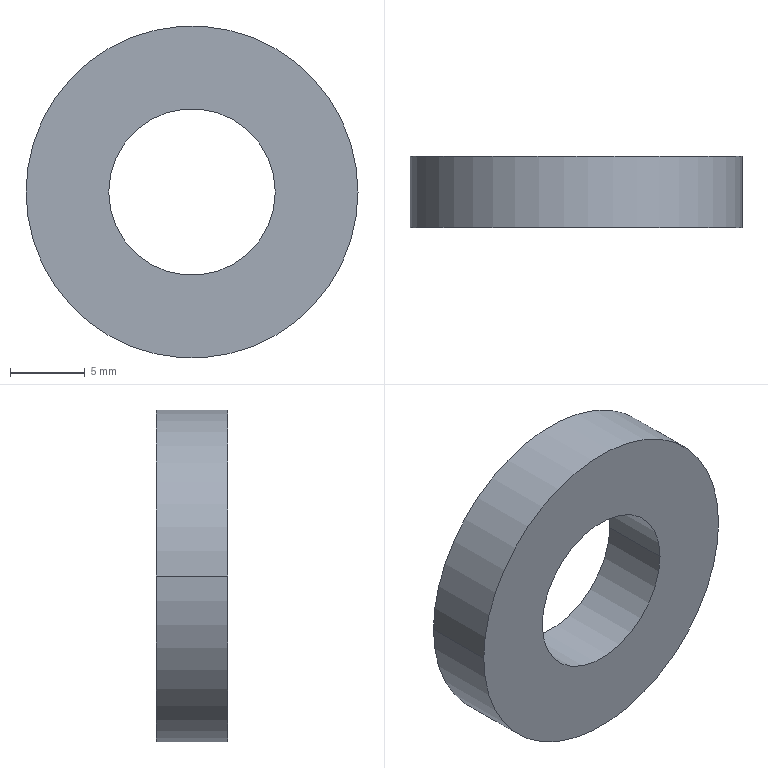Part | NX | features BREP 1 | 1 solid | 6 faces | box 22.225 x 4.763 x 22.225 mm | volume 1383 mm3 | cylinder 4 | plane 2 | commonest cylinder face diameters 11.151 x2 22.225 x2
STEP:
#1=CARTESIAN_POINT('',(-11.113,0.,0.));
#2=VERTEX_POINT('',#1);
#3=CARTESIAN_POINT('',(11.113,0.,0.));
#4=VERTEX_POINT('',#3);
#5=CARTESIAN_POINT('',(0.,0.,0.));
#6=DIRECTION('',(0.,1.,0.));
#7=DIRECTION('',(-1.,0.,0.));
#8=AXIS2_PLACEMENT_3D('',#5,#6,#7);
#9=CIRCLE('',#8,11.113);
#10=EDGE_CURVE('',#2,#4,#9,.T.);
#11=ORIENTED_EDGE('',*,*,#10,.F.);
#12=CARTESIAN_POINT('',(0.,0.,0.));
#13=DIRECTION('',(0.,1.,0.));
#14=DIRECTION('',(1.,0.,0.));
#15=AXIS2_PLACEMENT_3D('',#12,#13,#14);
#16=CIRCLE('',#15,11.113);
#17=EDGE_CURVE('',#4,#2,#16,.T.);
#18=ORIENTED_EDGE('',*,*,#17,.F.);
#19=EDGE_LOOP('',(#11,#18));
#20=FACE_BOUND('',#19,.T.);
#21=CARTESIAN_POINT('',(-5.575,0.,0.));
#22=VERTEX_POINT('',#21);
#23=CARTESIAN_POINT('',(5.575,0.,0.));
#24=VERTEX_POINT('',#23);
#25=CARTESIAN_POINT('',(0.,0.,0.));
#26=DIRECTION('',(0.,-1.,0.));
#27=DIRECTION('',(-1.,0.,0.));
#28=AXIS2_PLACEMENT_3D('',#25,#26,#27);
#29=CIRCLE('',#28,5.575);
#30=EDGE_CURVE('',#22,#24,#29,.T.);
#31=ORIENTED_EDGE('',*,*,#30,.F.);
#32=CARTESIAN_POINT('',(0.,0.,0.));
#33=DIRECTION('',(0.,-1.,0.));
#34=DIRECTION('',(1.,0.,0.));
#35=AXIS2_PLACEMENT_3D('',#32,#33,#34);
#36=CIRCLE('',#35,5.575);
#37=EDGE_CURVE('',#24,#22,#36,.T.);
#38=ORIENTED_EDGE('',*,*,#37,.F.);
#39=EDGE_LOOP('',(#31,#38));
#40=FACE_BOUND('',#39,.T.);
#41=CARTESIAN_POINT('',(0.,0.,0.));
#42=DIRECTION('',(0.,1.,0.));
#43=DIRECTION('',(1.,0.,0.));
#44=AXIS2_PLACEMENT_3D('',#41,#42,#43);
#45=PLANE('',#44);
#46=ADVANCED_FACE('',(#20,#40),#45,.F.);
#47=CARTESIAN_POINT('',(-11.113,4.763,0.));
#48=VERTEX_POINT('',#47);
#49=CARTESIAN_POINT('',(-11.113,0.,0.));
#50=DIRECTION('',(0.,1.,0.));
#51=VECTOR('',#50,1000.);
#52=LINE('',#49,#51);
#53=EDGE_CURVE('',#2,#48,#52,.T.);
#54=ORIENTED_EDGE('',*,*,#53,.T.);
#55=CARTESIAN_POINT('',(11.113,4.763,0.));
#56=VERTEX_POINT('',#55);
#57=CARTESIAN_POINT('',(0.,4.763,0.));
#58=DIRECTION('',(0.,1.,0.));
#59=DIRECTION('',(1.,0.,0.));
#60=AXIS2_PLACEMENT_3D('',#57,#58,#59);
#61=CIRCLE('',#60,11.113);
#62=EDGE_CURVE('',#56,#48,#61,.T.);
#63=ORIENTED_EDGE('',*,*,#62,.F.);
#64=CARTESIAN_POINT('',(11.113,0.,0.));
#65=DIRECTION('',(0.,1.,0.));
#66=VECTOR('',#65,1000.);
#67=LINE('',#64,#66);
#68=EDGE_CURVE('',#4,#56,#67,.T.);
#69=ORIENTED_EDGE('',*,*,#68,.F.);
#70=ORIENTED_EDGE('',*,*,#17,.T.);
#71=EDGE_LOOP('',(#54,#63,#69,#70));
#72=FACE_BOUND('',#71,.T.);
#73=CARTESIAN_POINT('',(0.,0.,0.));
#74=DIRECTION('',(0.,1.,0.));
#75=DIRECTION('',(1.,0.,0.));
#76=AXIS2_PLACEMENT_3D('',#73,#74,#75);
#77=CYLINDRICAL_SURFACE('',#76,11.113);
#78=ADVANCED_FACE('',(#72),#77,.T.);
#79=ORIENTED_EDGE('',*,*,#68,.T.);
#80=CARTESIAN_POINT('',(0.,4.763,0.));
#81=DIRECTION('',(0.,1.,0.));
#82=DIRECTION('',(-1.,0.,0.));
#83=AXIS2_PLACEMENT_3D('',#80,#81,#82);
#84=CIRCLE('',#83,11.113);
#85=EDGE_CURVE('',#48,#56,#84,.T.);
#86=ORIENTED_EDGE('',*,*,#85,.F.);
#87=ORIENTED_EDGE('',*,*,#53,.F.);
#88=ORIENTED_EDGE('',*,*,#10,.T.);
#89=EDGE_LOOP('',(#79,#86,#87,#88));
#90=FACE_BOUND('',#89,.T.);
#91=CARTESIAN_POINT('',(0.,0.,0.));
#92=DIRECTION('',(0.,1.,0.));
#93=DIRECTION('',(1.,0.,0.));
#94=AXIS2_PLACEMENT_3D('',#91,#92,#93);
#95=CYLINDRICAL_SURFACE('',#94,11.113);
#96=ADVANCED_FACE('',(#90),#95,.T.);
#97=ORIENTED_EDGE('',*,*,#85,.T.);
#98=ORIENTED_EDGE('',*,*,#62,.T.);
#99=EDGE_LOOP('',(#97,#98));
#100=FACE_BOUND('',#99,.T.);
#101=CARTESIAN_POINT('',(-5.575,4.763,0.));
#102=VERTEX_POINT('',#101);
#103=CARTESIAN_POINT('',(5.575,4.763,0.));
#104=VERTEX_POINT('',#103);
#105=CARTESIAN_POINT('',(0.,4.763,0.));
#106=DIRECTION('',(0.,-1.,0.));
#107=DIRECTION('',(-1.,0.,0.));
#108=AXIS2_PLACEMENT_3D('',#105,#106,#107);
#109=CIRCLE('',#108,5.575);
#110=EDGE_CURVE('',#102,#104,#109,.T.);
#111=ORIENTED_EDGE('',*,*,#110,.T.);
#112=CARTESIAN_POINT('',(0.,4.763,0.));
#113=DIRECTION('',(0.,-1.,0.));
#114=DIRECTION('',(1.,0.,0.));
#115=AXIS2_PLACEMENT_3D('',#112,#113,#114);
#116=CIRCLE('',#115,5.575);
#117=EDGE_CURVE('',#104,#102,#116,.T.);
#118=ORIENTED_EDGE('',*,*,#117,.T.);
#119=EDGE_LOOP('',(#111,#118));
#120=FACE_BOUND('',#119,.T.);
#121=CARTESIAN_POINT('',(0.,4.763,0.));
#122=DIRECTION('',(0.,1.,0.));
#123=DIRECTION('',(1.,0.,0.));
#124=AXIS2_PLACEMENT_3D('',#121,#122,#123);
#125=PLANE('',#124);
#126=ADVANCED_FACE('',(#100,#120),#125,.T.);
#127=CARTESIAN_POINT('',(-5.575,4.763,0.));
#128=DIRECTION('',(0.,-1.,0.));
#129=VECTOR('',#128,1000.);
#130=LINE('',#127,#129);
#131=EDGE_CURVE('',#102,#22,#130,.T.);
#132=ORIENTED_EDGE('',*,*,#131,.F.);
#133=ORIENTED_EDGE('',*,*,#117,.F.);
#134=CARTESIAN_POINT('',(5.575,4.763,0.));
#135=DIRECTION('',(0.,-1.,0.));
#136=VECTOR('',#135,1000.);
#137=LINE('',#134,#136);
#138=EDGE_CURVE('',#104,#24,#137,.T.);
#139=ORIENTED_EDGE('',*,*,#138,.T.);
#140=ORIENTED_EDGE('',*,*,#37,.T.);
#141=EDGE_LOOP('',(#132,#133,#139,#140));
#142=FACE_BOUND('',#141,.T.);
#143=CARTESIAN_POINT('',(0.,4.763,0.));
#144=DIRECTION('',(0.,-1.,0.));
#145=DIRECTION('',(1.,0.,0.));
#146=AXIS2_PLACEMENT_3D('',#143,#144,#145);
#147=CYLINDRICAL_SURFACE('',#146,5.575);
#148=ADVANCED_FACE('',(#142),#147,.F.);
#149=ORIENTED_EDGE('',*,*,#138,.F.);
#150=ORIENTED_EDGE('',*,*,#110,.F.);
#151=ORIENTED_EDGE('',*,*,#131,.T.);
#152=ORIENTED_EDGE('',*,*,#30,.T.);
#153=EDGE_LOOP('',(#149,#150,#151,#152));
#154=FACE_BOUND('',#153,.T.);
#155=CARTESIAN_POINT('',(0.,4.763,0.));
#156=DIRECTION('',(0.,-1.,0.));
#157=DIRECTION('',(1.,0.,0.));
#158=AXIS2_PLACEMENT_3D('',#155,#156,#157);
#159=CYLINDRICAL_SURFACE('',#158,5.575);
#160=ADVANCED_FACE('',(#154),#159,.F.);
#161=CLOSED_SHELL('',(#46,#78,#96,#126,#148,#160));
#162=MANIFOLD_SOLID_BREP('',#161);
#163=(LENGTH_UNIT()NAMED_UNIT(*)SI_UNIT(.MILLI.,.METRE.));
#164=UNCERTAINTY_MEASURE_WITH_UNIT(LENGTH_MEASURE(0.00001),#163,'','');
#165=(NAMED_UNIT(*)PLANE_ANGLE_UNIT()SI_UNIT($,.RADIAN.));
#166=(NAMED_UNIT(*)SI_UNIT($,.STERADIAN.)SOLID_ANGLE_UNIT());
#167=(GEOMETRIC_REPRESENTATION_CONTEXT(3)GLOBAL_UNCERTAINTY_ASSIGNED_CONTEXT((#164))GLOBAL_UNIT_ASSIGNED_CONTEXT((#163,#165,#166))REPRESENTATION_CONTEXT('',''));
#168=ADVANCED_BREP_SHAPE_REPRESENTATION('',(#162),#167);